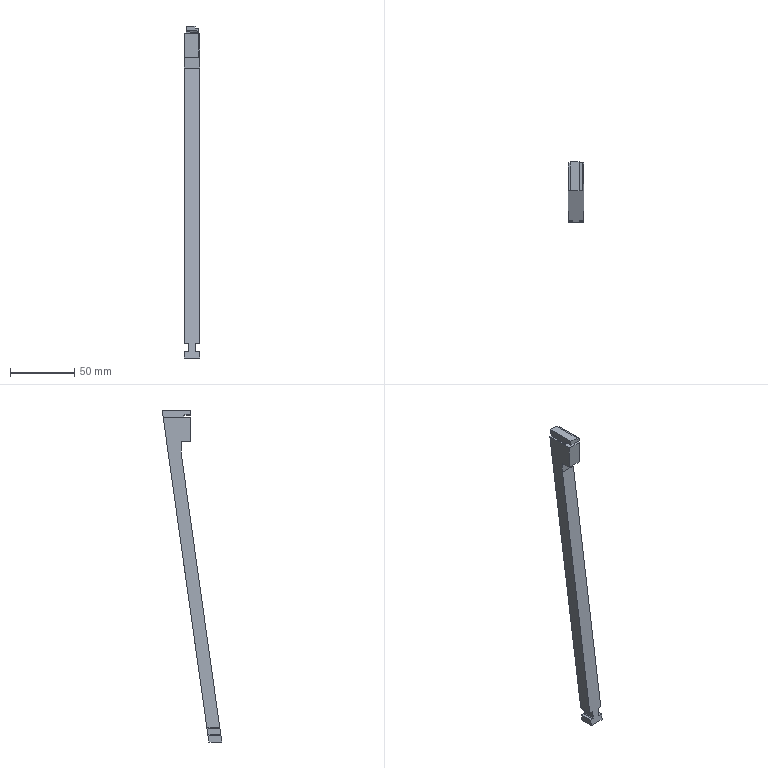Part | Creo | 1 solid | 109 faces | box 12 x 46.477 x 258.85 mm | volume 33467 mm3 | other 53 | plane 50 | cylinder 6 | commonest cylinder face diameters 1 x4 2 x1 23.149 x1